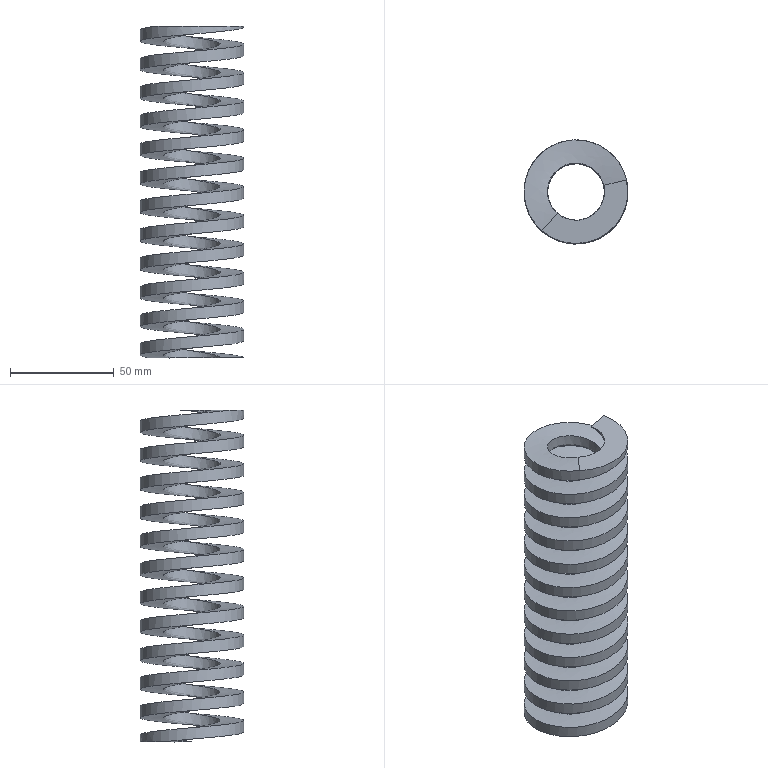Part | NX | features solid 2 | 1 solid | 5 faces | box 50.009 x 50.008 x 160 mm | volume 82264 mm3 | plane 2 | spline 2 | cylinder 1 | commonest cylinder face diameters 50 x1